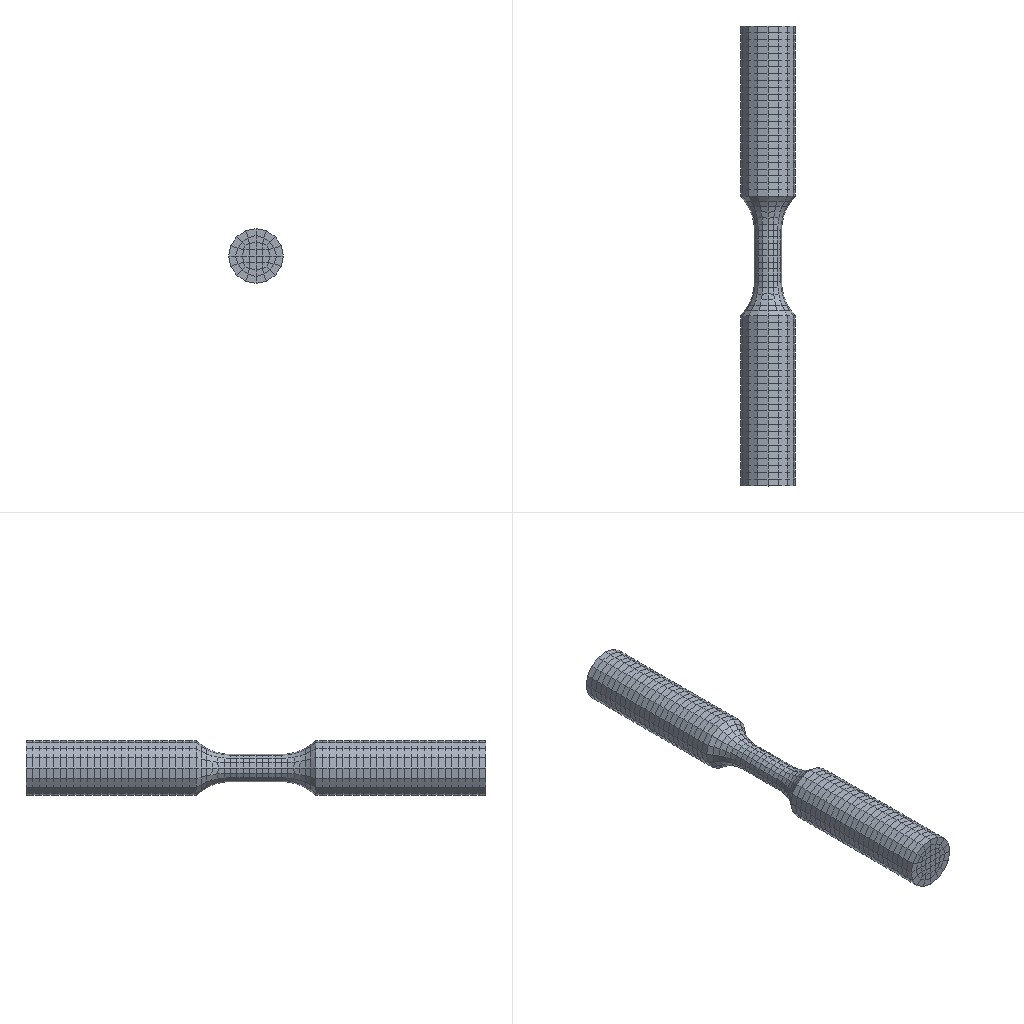Simulation study | abaqus
Set-up summary:
category,name,step,type,value,unit,region
solver,abaqus,,Abaqus/CAE 2024
units,mm-N-s-tonne (MPa),,inferred,E=200000 density=7.85e-09
analysis,Step-1,,dynamic explicit,nlgeom=True; time_period=0.1
mesh,nodes,,,3562
mesh,elements,,,2880
element_type,C3D8R,,,2880
material,Material-1-Copy,,E,200000
material,Material-1-Copy,,nu,0.3
material,Material-1-Copy,,density,7.85e-09
material,Material-1-Copy,,yield,1080
material,Material-1-Copy,,behaviors,plastic; damage initiation; damage evolution; damage initiation; damage evolution
material,Material-1-Copy-Copy,,E,200000
material,Material-1-Copy-Copy,,nu,0.3
material,Material-1-Copy-Copy,,density,7.85e-09
material,Material-1-Copy-Copy,,yield,1080
material,Material-1-Copy-Copy,,behaviors,plastic; damage initiation; damage evolution; damage initiation; damage evolution
section,Material-1-Copy-Copy,,solid section,,,_PickedSet8
bc,BC-1,Step-1,encastre,[dofs=ENCASTRE],,_PickedSet19
bc,BC-2,Step-1,fixed,"[dofs=rx,ry,rz,x,z n=5]",,_PickedSet20
bc,BC-2,Step-1,displacement,10 [dofs=y],,_PickedSet20
constraint,coupling,,,1
Abaqus input file, long lists of numbers shortened:
*Heading
** Job name: deck Model name: 1010
** Generated by: Abaqus/CAE 2024
*Preprint, echo=NO, model=NO, history=NO, contact=NO
**
** PARTS
**
*Part, name=Part-p
*Node
      1,           0.,          75.,           4.
      2,           0.,          75.,           0.
** (3559 more lines like these left out)
*Element, type=C3D8R
 1,  480,  481, 2019, 2014,   31,   32,  463,  462
 2,  481,   41,  466, 2019,   32,    1,   33,  463
** (2878 more lines like these left out)
*Nset, nset=_PickedSet8, internal, generate
    1,  3561,     1
*Elset, elset=_PickedSet8, internal, generate
    1,  2880,     1
** Section: Section-2
*Solid Section, elset=_PickedSet8, controls=EC-1, material=Material-1-Copy-Copy
,
*End Part
**
**
** ASSEMBLY
**
*Assembly, name=Assembly
**
*Instance, name=Part-p-1, part=Part-p
*End Instance
**
*Node
      1,           0.,         135., 7.776507e-15
*Nset, nset=_PickedSet18, internal
 1,
*Nset, nset=_PickedSet19, internal, instance=Part-p-1
   22,   23,   24,   25,   26,   27,   28,   29,  326,  327,  328,  329,  330,  331,  332,  333
  334,  335,  336,  337,  338,  339,  340,  341,  342,  343,  344,  345,  346,  347,  348,  349
** (24 more lines like these left out)
*Elset, elset=_PickedSet19, internal, instance=Part-p-1
 1698, 1700, 1702, 1704, 1706, 1708, 1710, 1712, 1714, 1716, 1718, 1720, 1722, 1724, 1726, 1728
 1730, 1732, 1734, 1736, 1738, 1740, 1742, 1744, 1746, 1748, 1750, 1752, 1754, 1756, 1758, 1760
** (23 more lines like these left out)
*Nset, nset=_PickedSet20, internal
 1,
*Elset, elset=__PickedSurf17_S4, internal, instance=Part-p-1
  202,  204,  218,  220,  222,  224,  226,  228,  230,  232,  234,  236,  238,  240,  242,  244
  246,  248,  250,  252,  254,  256,  258,  260,  262,  264,  266,  268,  270,  272,  274,  276
** (11 more lines like these left out)
*Elset, elset=__PickedSurf17_S3, internal, instance=Part-p-1
  205,  206,  425,  426,  427,  428,  429,  430,  431,  432,  433,  434,  435,  436,  437,  438
  439,  440,  441,  442,  443,  444,  445,  446,  447,  448,  473,  474,  475,  476,  477,  478
** (11 more lines like these left out)
*Surface, type=ELEMENT, name=_PickedSurf17, internal
__PickedSurf17_S4, S4
__PickedSurf17_S3, S3
** Constraint: Constraint-1
*Coupling, constraint name=Constraint-1, ref node=_PickedSet18, surface=_PickedSurf17
*Kinematic
*End Assembly
**
** ELEMENT CONTROLS
**
*Section Controls, name=EC-1, ELEMENT DELETION=YES
1., 1., 1.
*Amplitude, name=Amp-1
             0.,              0.,             0.1,              1.
**
** MATERIALS
**
*Material, name=Material-1-Copy
*Damage Initiation, criterion=DUCTILE
  27.141,  -1.,  0.1
  10.761, -0.5,  0.1
  4.266,   0.,  0.1
  1.691,  0.5,  0.1
 0.6706,   1.,  0.1
 0.2659,  1.5,  0.1
 0.1054,   2.,  0.1
*Damage Evolution, type=DISPLACEMENT
1.,
*Damage Initiation, criterion=SHEAR
  27.141,  -1.,  0.1
  10.761, -0.5,  0.1
  4.266,   0.,  0.1
  1.691,  0.5,  0.1
 0.6706,   1.,  0.1
 0.2659,  1.5,  0.1
 0.1054,   2.,  0.1
*Damage Evolution, type=DISPLACEMENT
1.,
*Density
 7.85e-09,
*Elastic
200000., 0.3
*Plastic
1080.,      0.
1318., 0.03015
*Material, name=Material-1-Copy-Copy
*Damage Initiation, criterion=DUCTILE
  27.141,  -1.,  0.1
  10.761, -0.5,  0.1
  4.266,   0.,  0.1
  1.691,  0.5,  0.1
 0.6706,   1.,  0.1
 0.2659,  1.5,  0.1
 0.1054,   2.,  0.1
*Damage Evolution, type=DISPLACEMENT
 0.1,
*Damage Initiation, criterion=SHEAR
  27.141,  -1.,  0.1
  10.761, -0.5,  0.1
  4.266,   0.,  0.1
  1.691,  0.5,  0.1
 0.6706,   1.,  0.1
 0.2659,  1.5,  0.1
 0.1054,   2.,  0.1
*Damage Evolution, type=DISPLACEMENT
 0.1,
*Density
 7.85e-09,
*Elastic
200000., 0.3
*Plastic
1080.,      0.
1318., 0.03015
** ----------------------------------------------------------------
**
** STEP: Step-1
**
*Step, name=Step-1, nlgeom=YES
*Dynamic, Explicit
, 0.1
*Bulk Viscosity
0.06, 1.2
** Mass Scaling: Semi-Automatic
**               Whole Model
*Fixed Mass Scaling, factor=100.
**
** BOUNDARY CONDITIONS
**
** Name: BC-1 Type: Symmetry/Antisymmetry/Encastre
*Boundary
_PickedSet19, ENCASTRE
** Name: BC-2 Type: Displacement/Rotation
*Boundary, amplitude=Amp-1
_PickedSet20, 1, 1
_PickedSet20, 2, 2, 10.
_PickedSet20, 3, 3
_PickedSet20, 4, 4
_PickedSet20, 5, 5
_PickedSet20, 6, 6
**
** OUTPUT REQUESTS
**
*Restart, write, number interval=1, time marks=NO
**
** FIELD OUTPUT: F-Output-1
**
*Output, field, number interval=40
*Node Output
A, RF, U, V
*Element Output, directions=YES
EVF, LE, PE, PEEQ, PEEQVAVG, PEVAVG, S, SDEG, STATUS, SVAVG
*Contact Output
CSTRESS,
**
** HISTORY OUTPUT: H-Output-1
**
*Output, history, variable=PRESELECT
*End Step
Results summary:
result,odb.job_status,,,JOB_STATUS_COMPLETED_SUCCESSFULLY,"consistent, unstated (Abaqus has no unit system)"
result,steps[0].procedure,Step-1,,"*DYNAMIC, EXPLICIT","consistent, unstated (Abaqus has no unit system)"
result,steps[0].time_period,Step-1,,0.1,"consistent, unstated (Abaqus has no unit system)"
result,steps[0].n_frames,Step-1,,41,"consistent, unstated (Abaqus has no unit system)"
result,steps[0].last_frame.id,Step-1,,62070,"consistent, unstated (Abaqus has no unit system)"
result,steps[0].last_frame.value,Step-1,,0.1,"consistent, unstated (Abaqus has no unit system)"
result,steps[0].last_frame.description,Step-1,,Increment     62070: Step Time =   0.1,"consistent, unstated (Abaqus has no unit system)"
result,steps[0].completed,Step-1,,True,"consistent, unstated (Abaqus has no unit system)"
result,steps[0].max_U_magnitude,Step-1,,10.002,"consistent, unstated (Abaqus has no unit system)"
result,steps[0].max_S_mises,Step-1,,497.859,"consistent, unstated (Abaqus has no unit system)"
result,steps[0].RF_sum[1],Step-1,,3.123,"consistent, unstated (Abaqus has no unit system)"
result,steps[0].RF_sum[2],Step-1,,176.414,"consistent, unstated (Abaqus has no unit system)"
result,steps[0].RF_sum[3],Step-1,,-12.726,"consistent, unstated (Abaqus has no unit system)"
result,steps[0].diagnostic.n_increments,Step-1,,41,"consistent, unstated (Abaqus has no unit system)"